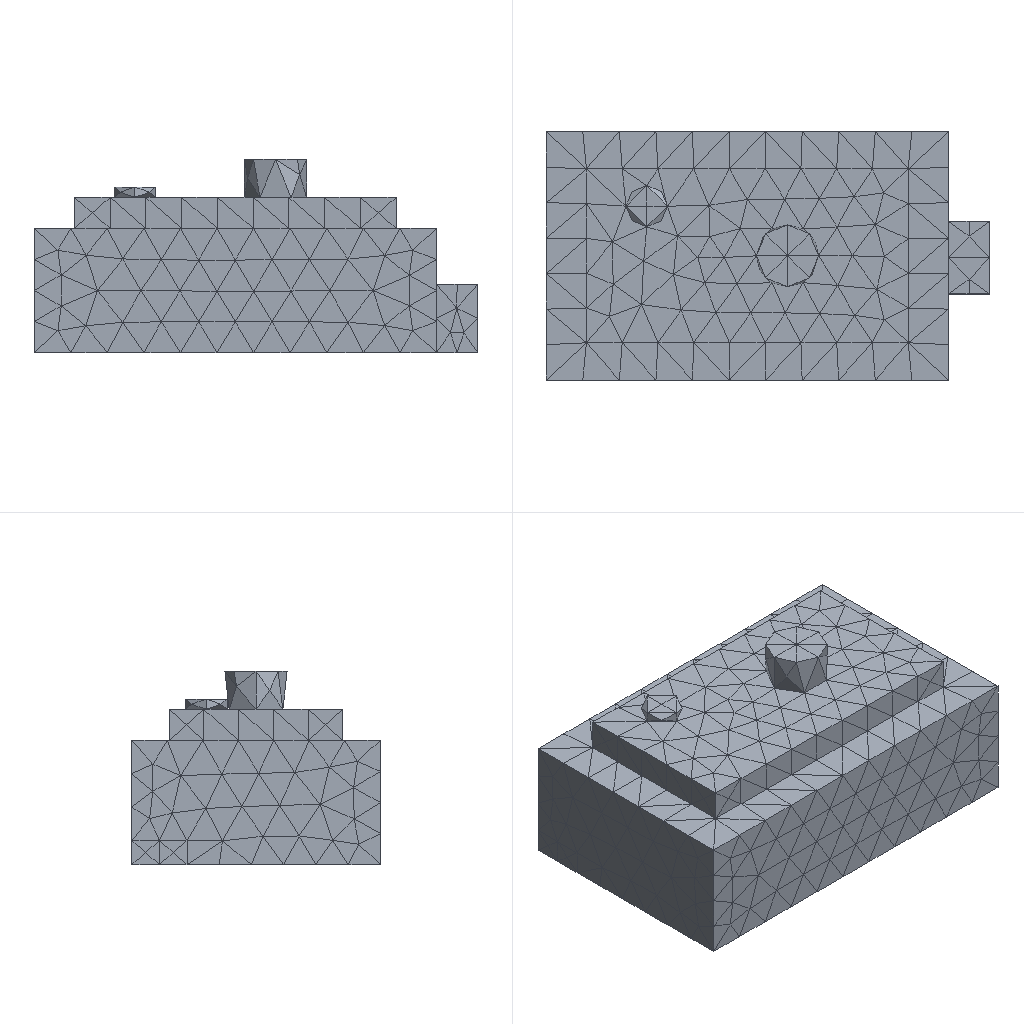Simulation study | ansys mapdl
Set-up summary:
category,name,step,type,value,unit,region
solver,ansys_mapdl
units,mm-N-s-tonne (MPa),,inferred,E=210000 density=
analysis,model,,static
mesh,nodes,,,4664
mesh,elements,,,2784
element_type,SOLID187,,,2784
material,mat 1,,E,210000
material,mat 1,,nu,0.3
load,,model,body load temp,,,all
load,,model,force,"1000 [dir=(0, 0, -1) n=106]",,node list
bc,,model,fixed,"[dofs=UX,UY,UZ n=5191]",,node list
Ansys APDL input file, long lists of numbers shortened:
/COM,ANSYS RELEASE 2026 R1           BUILD 26.1      UP20260202       09:11:06
/PREP7
/NOPR
/TITLE,2
ANTYPE, 0
*IF,_CDRDOFF,EQ,1,THEN     !if solid model was read in
_CDRDOFF=             !reset flag, numoffs already performed
*ELSE              !offset database for the following FE model
NUMOFF,NODE,     4664
NUMOFF,ELEM,     2784
NUMOFF,MAT ,        1
NUMOFF,TYPE,        1
*ENDIF
*SET,_RETURN ,  0.
*SET,_STATUS ,  0.
*SET,_UIQR   ,  106.
*SET,__FLOATPARAMETER__,  4664.
DOF,DELETE
ETBLOCK,        1,        1
(2i9,19a9)
        1      187        0        0        0        0        0        0        0        0        0        0        0        0        0        0        0        0        0        0        0
       -1
NBLOCK,6,SOLID,      4664,      4664
(3i9,6e21.13e3)
        1        0        0-4.2300000000000E+001 3.6000000000000E+001 7.0000000000000E+000
! (4663 more lines like these left out)
N,UNBL,LOC,       -1,
EBLOCK,19,SOLID,      2784,      2784
(19i10)
         1         1         1         1         0         0         0         0        10         0         1      1799      1800       421      1801      2064      2065      2066      2067
! (5567 more lines like these left out)
        -1
MPTEMP,UNBL, 1, 1,  0.    ,
MPDATA,UNBL, 1,EX  ,       1, 1,  210000.000    ,
MPTEMP,UNBL, 1, 1,  0.    ,
MPDATA,UNBL, 1,NUXY,       1, 1, 0.3    ,
MPTEMP,UNBL, 1, 1,  0.    ,
MPDATA,UNBL, 1,PRXY,       1, 1, 0.3    ,
EXTOPT,ATTR,      0,      0,      0
EXTOPT,ESIZE,  0,  0.
EXTOPT,ACLEAR,      0
TREF,  0.
IRLF,  0
BFUNIF,TEMP,_TINY
ACEL,  0.    ,  0.    ,  0.
OMEGA,  0.    ,  0.    ,  0.
DOMEGA,  0.    ,  0.    ,  0.
CGLOC,  0.    ,  0.    ,  0.
CGOMEGA,  0.    ,  0.    ,  0.
DCGOMG,  0.    ,  0.    ,  0.
KUSE,     0
TIME,  0.
ALPHAD,  0.
BETAD,  0.
DMPRAT,  0.
DMPSTR,  0.
CRPLIM, 0.1    ,   0
CRPLIM,  0.    ,   1
NCNV,     0, 1.000000000E+12,     0,  0.    ,  0.
NEQIT,     0
ERESX,DEFA
DBLOCK,      5191
(i9,a6,2(pg16.9))
        1  UX    0.00000000      0.00000000
! (5190 more lines like these left out)
       -1
FBLOCK,       106
(i9,a6,2(pg16.9))
      878  FZ   -9.43396226      0.00000000
! (105 more lines like these left out)
       -1
/GO
FINISH
Results summary:
result,analysis_type_db,,,static,unstated
result,n_sets,,,1,unstated
result,load_steps[0].set,load_step=1,,1,unstated
result,load_steps[0].substep,load_step=1,,1,unstated
result,load_steps[0].time,load_step=1,,1,unstated
result,load_steps[0].freq,load_step=1,,1,unstated
result,load_steps[0].max_usum,load_step=1,,0.0002773,unstated
result,load_steps[0].max_seqv,load_step=1,,12.182,unstated
result,load_steps[0].reaction_sum.FX,load_step=1,,3.93463e-12,unstated
result,load_steps[0].reaction_sum.FY,load_step=1,,-2.74945e-11,unstated
result,load_steps[0].reaction_sum.FZ,load_step=1,,1000,unstated
result,load_steps[0].reaction_sum.MX,load_step=1,,0,unstated
result,load_steps[0].reaction_sum.MY,load_step=1,,0,unstated
result,load_steps[0].reaction_sum.MZ,load_step=1,,0,unstated
result,convergence,,,results present for all listed sets,unstated